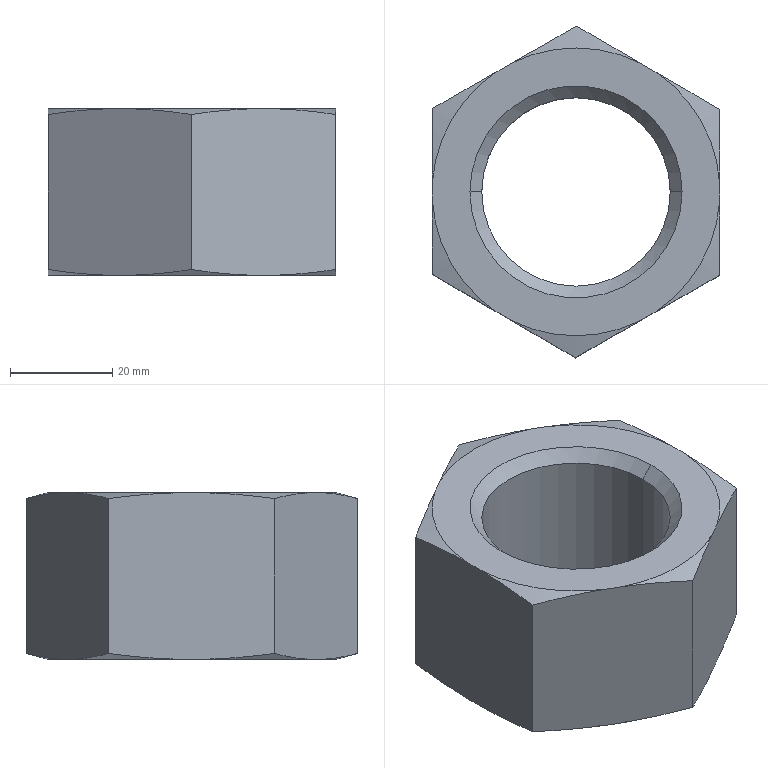Part | SolidWorks | features Cut 2, Chamfer 1, Extrusion 1 | 1 solid | 26 faces | box 56.219 x 64.769 x 32.544 mm | volume 53250 mm3 | cone 16 | plane 8 | cylinder 2 | commonest cylinder face diameters 36.8 x2
STEP:
#1=CARTESIAN_POINT('',(-18.4,0.,30.237));
#2=VERTEX_POINT('',#1);
#3=CARTESIAN_POINT('',(18.4,0.,30.237));
#4=VERTEX_POINT('',#3);
#5=CARTESIAN_POINT('',(0.,0.,30.237));
#6=DIRECTION('',(0.,0.,1.));
#7=DIRECTION('',(-1.,0.,0.));
#8=AXIS2_PLACEMENT_3D('',#5,#6,#7);
#9=CIRCLE('',#8,18.4);
#10=EDGE_CURVE('',#2,#4,#9,.T.);
#11=ORIENTED_EDGE('',*,*,#10,.F.);
#12=CARTESIAN_POINT('',(-20.707,0.,32.544));
#13=VERTEX_POINT('',#12);
#14=CARTESIAN_POINT('',(-18.4,0.,30.237));
#15=DIRECTION('',(-0.7071,0.,0.7071));
#16=VECTOR('',#15,1000.);
#17=LINE('',#14,#16);
#18=EDGE_CURVE('',#2,#13,#17,.T.);
#19=ORIENTED_EDGE('',*,*,#18,.T.);
#20=CARTESIAN_POINT('',(20.707,0.,32.544));
#21=VERTEX_POINT('',#20);
#22=CARTESIAN_POINT('',(0.,0.,32.544));
#23=DIRECTION('',(0.,0.,-1.));
#24=DIRECTION('',(-1.,0.,0.));
#25=AXIS2_PLACEMENT_3D('',#22,#23,#24);
#26=CIRCLE('',#25,20.707);
#27=EDGE_CURVE('',#21,#13,#26,.T.);
#28=ORIENTED_EDGE('',*,*,#27,.F.);
#29=CARTESIAN_POINT('',(18.4,0.,30.237));
#30=DIRECTION('',(0.7071,0.,0.7071));
#31=VECTOR('',#30,1000.);
#32=LINE('',#29,#31);
#33=EDGE_CURVE('',#4,#21,#32,.T.);
#34=ORIENTED_EDGE('',*,*,#33,.F.);
#35=EDGE_LOOP('',(#11,#19,#28,#34));
#36=FACE_OUTER_BOUND('',#35,.T.);
#37=CARTESIAN_POINT('',(0.,0.,30.237));
#38=DIRECTION('',(0.,0.,1.));
#39=DIRECTION('',(1.,0.,0.));
#40=AXIS2_PLACEMENT_3D('',#37,#38,#39);
#41=CONICAL_SURFACE('',#40,18.4,0.7854);
#42=ADVANCED_FACE('',(#36),#41,.F.);
#43=CARTESIAN_POINT('',(18.4,0.,2.307));
#44=VERTEX_POINT('',#43);
#45=CARTESIAN_POINT('',(-18.4,0.,2.307));
#46=VERTEX_POINT('',#45);
#47=CARTESIAN_POINT('',(0.,0.,2.307));
#48=DIRECTION('',(0.,0.,-1.));
#49=DIRECTION('',(-1.,0.,0.));
#50=AXIS2_PLACEMENT_3D('',#47,#48,#49);
#51=CIRCLE('',#50,18.4);
#52=EDGE_CURVE('',#44,#46,#51,.T.);
#53=ORIENTED_EDGE('',*,*,#52,.F.);
#54=CARTESIAN_POINT('',(20.707,0.,0.));
#55=VERTEX_POINT('',#54);
#56=CARTESIAN_POINT('',(20.707,0.,0.));
#57=DIRECTION('',(0.7071,0.,-0.7071));
#58=VECTOR('',#57,1000.);
#59=LINE('',#56,#58);
#60=EDGE_CURVE('',#44,#55,#59,.T.);
#61=ORIENTED_EDGE('',*,*,#60,.T.);
#62=CARTESIAN_POINT('',(-20.707,0.,0.));
#63=VERTEX_POINT('',#62);
#64=CARTESIAN_POINT('',(0.,0.,0.));
#65=DIRECTION('',(0.,0.,1.));
#66=DIRECTION('',(-1.,0.,0.));
#67=AXIS2_PLACEMENT_3D('',#64,#65,#66);
#68=CIRCLE('',#67,20.707);
#69=EDGE_CURVE('',#63,#55,#68,.T.);
#70=ORIENTED_EDGE('',*,*,#69,.F.);
#71=CARTESIAN_POINT('',(-20.707,0.,0.));
#72=DIRECTION('',(-0.7071,0.,-0.7071));
#73=VECTOR('',#72,1000.);
#74=LINE('',#71,#73);
#75=EDGE_CURVE('',#46,#63,#74,.T.);
#76=ORIENTED_EDGE('',*,*,#75,.F.);
#77=EDGE_LOOP('',(#53,#61,#70,#76));
#78=FACE_OUTER_BOUND('',#77,.T.);
#79=CARTESIAN_POINT('',(0.,0.,0.));
#80=DIRECTION('',(0.,0.,-1.));
#81=DIRECTION('',(-1.,0.,0.));
#82=AXIS2_PLACEMENT_3D('',#79,#80,#81);
#83=CONICAL_SURFACE('',#82,20.707,0.7854);
#84=ADVANCED_FACE('',(#78),#83,.F.);
#85=ORIENTED_EDGE('',*,*,#10,.T.);
#86=CARTESIAN_POINT('',(18.4,0.,32.544));
#87=DIRECTION('',(0.,0.,-1.));
#88=VECTOR('',#87,1000.);
#89=LINE('',#86,#88);
#90=EDGE_CURVE('',#4,#44,#89,.T.);
#91=ORIENTED_EDGE('',*,*,#90,.T.);
#92=ORIENTED_EDGE('',*,*,#52,.T.);
#93=CARTESIAN_POINT('',(-18.4,0.,32.544));
#94=DIRECTION('',(0.,0.,-1.));
#95=VECTOR('',#94,1000.);
#96=LINE('',#93,#95);
#97=EDGE_CURVE('',#2,#46,#96,.T.);
#98=ORIENTED_EDGE('',*,*,#97,.F.);
#99=EDGE_LOOP('',(#85,#91,#92,#98));
#100=FACE_OUTER_BOUND('',#99,.T.);
#101=CARTESIAN_POINT('',(0.,0.,32.544));
#102=DIRECTION('',(0.,0.,-1.));
#103=DIRECTION('',(-1.,0.,0.));
#104=AXIS2_PLACEMENT_3D('',#101,#102,#103);
#105=CYLINDRICAL_SURFACE('',#104,18.4);
#106=ADVANCED_FACE('',(#100),#105,.F.);
#107=CARTESIAN_POINT('',(28.11,16.082,31.396));
#108=VERTEX_POINT('',#107);
#109=CARTESIAN_POINT('',(15.62,23.359,32.544));
#110=VERTEX_POINT('',#109);
#111=CARTESIAN_POINT('',(28.11,16.082,31.396));
#112=CARTESIAN_POINT('',(26.042,17.287,31.716));
#113=CARTESIAN_POINT('',(23.968,18.495,31.984));
#114=CARTESIAN_POINT('',(19.806,20.92,32.378));
#115=CARTESIAN_POINT('',(17.718,22.137,32.504));
#116=CARTESIAN_POINT('',(15.62,23.359,32.544));
#117=B_SPLINE_CURVE_WITH_KNOTS('',3,(#111,#112,#113,#114,#115,#116),.UNSPECIFIED.,.F.,.F.,(4,2,4),(0.03192,0.03916,0.04641),.UNSPECIFIED.);
#118=EDGE_CURVE('',#108,#110,#117,.T.);
#119=ORIENTED_EDGE('',*,*,#118,.F.);
#120=CARTESIAN_POINT('',(28.11,16.082,1.148));
#121=VERTEX_POINT('',#120);
#122=CARTESIAN_POINT('',(28.11,16.082,32.544));
#123=DIRECTION('',(0.,0.,-1.));
#124=VECTOR('',#123,1000.);
#125=LINE('',#122,#124);
#126=EDGE_CURVE('',#108,#121,#125,.T.);
#127=ORIENTED_EDGE('',*,*,#126,.T.);
#128=CARTESIAN_POINT('',(15.62,23.359,0.));
#129=VERTEX_POINT('',#128);
#130=CARTESIAN_POINT('',(15.62,23.359,0.));
#131=CARTESIAN_POINT('',(16.657,22.754,0.0199));
#132=CARTESIAN_POINT('',(17.697,22.148,0.06046));
#133=CARTESIAN_POINT('',(19.781,20.934,0.1815));
#134=CARTESIAN_POINT('',(20.826,20.325,0.2621));
#135=CARTESIAN_POINT('',(23.961,18.499,0.5582));
#136=CARTESIAN_POINT('',(26.039,17.288,0.8271));
#137=CARTESIAN_POINT('',(28.11,16.082,1.148));
#138=B_SPLINE_CURVE_WITH_KNOTS('',3,(#130,#131,#132,#133,#134,#135,#136,#137),.UNSPECIFIED.,.F.,.F.,(4,2,2,4),(0.04982,0.05339,0.05695,0.06409),.UNSPECIFIED.);
#139=EDGE_CURVE('',#129,#121,#138,.T.);
#140=ORIENTED_EDGE('',*,*,#139,.F.);
#141=CARTESIAN_POINT('',(12.617,25.108,0.));
#142=VERTEX_POINT('',#141);
#143=CARTESIAN_POINT('',(28.11,16.082,0.));
#144=DIRECTION('',(-0.8641,0.5034,0.));
#145=VECTOR('',#144,1000.);
#146=LINE('',#143,#145);
#147=EDGE_CURVE('',#129,#142,#146,.T.);
#148=ORIENTED_EDGE('',*,*,#147,.T.);
#149=CARTESIAN_POINT('',(0.1274,32.385,1.148));
#150=VERTEX_POINT('',#149);
#151=CARTESIAN_POINT('',(0.1274,32.385,1.148));
#152=CARTESIAN_POINT('',(2.195,31.18,0.8275));
#153=CARTESIAN_POINT('',(4.269,29.972,0.5593));
#154=CARTESIAN_POINT('',(8.431,27.547,0.1653));
#155=CARTESIAN_POINT('',(10.519,26.33,0.04022));
#156=CARTESIAN_POINT('',(12.617,25.108,0.));
#157=B_SPLINE_CURVE_WITH_KNOTS('',3,(#151,#152,#153,#154,#155,#156),.UNSPECIFIED.,.F.,.F.,(4,2,4),(0.03188,0.03913,0.04637),.UNSPECIFIED.);
#158=EDGE_CURVE('',#150,#142,#157,.T.);
#159=ORIENTED_EDGE('',*,*,#158,.F.);
#160=CARTESIAN_POINT('',(0.1274,32.385,31.396));
#161=VERTEX_POINT('',#160);
#162=CARTESIAN_POINT('',(0.1274,32.385,32.544));
#163=DIRECTION('',(0.,0.,-1.));
#164=VECTOR('',#163,1000.);
#165=LINE('',#162,#164);
#166=EDGE_CURVE('',#161,#150,#165,.T.);
#167=ORIENTED_EDGE('',*,*,#166,.F.);
#168=CARTESIAN_POINT('',(12.617,25.108,32.544));
#169=VERTEX_POINT('',#168);
#170=CARTESIAN_POINT('',(12.617,25.108,32.544));
#171=CARTESIAN_POINT('',(11.58,25.713,32.524));
#172=CARTESIAN_POINT('',(10.54,26.318,32.483));
#173=CARTESIAN_POINT('',(8.456,27.532,32.362));
#174=CARTESIAN_POINT('',(7.411,28.141,32.282));
#175=CARTESIAN_POINT('',(4.277,29.967,31.986));
#176=CARTESIAN_POINT('',(2.198,31.178,31.717));
#177=CARTESIAN_POINT('',(0.1274,32.385,31.396));
#178=B_SPLINE_CURVE_WITH_KNOTS('',3,(#170,#171,#172,#173,#174,#175,#176,#177),.UNSPECIFIED.,.F.,.F.,(4,2,2,4),(0.04985,0.05342,0.05699,0.06413),.UNSPECIFIED.);
#179=EDGE_CURVE('',#169,#161,#178,.T.);
#180=ORIENTED_EDGE('',*,*,#179,.F.);
#181=CARTESIAN_POINT('',(28.11,16.082,32.544));
#182=DIRECTION('',(-0.8641,0.5034,0.));
#183=VECTOR('',#182,1000.);
#184=LINE('',#181,#183);
#185=EDGE_CURVE('',#110,#169,#184,.T.);
#186=ORIENTED_EDGE('',*,*,#185,.F.);
#187=EDGE_LOOP('',(#119,#127,#140,#148,#159,#167,#180,#186));
#188=FACE_OUTER_BOUND('',#187,.T.);
#189=CARTESIAN_POINT('',(28.11,16.082,32.544));
#190=DIRECTION('',(-0.5034,-0.8641,0.));
#191=DIRECTION('',(0.8641,-0.5034,0.));
#192=AXIS2_PLACEMENT_3D('',#189,#190,#191);
#193=PLANE('',#192);
#194=ADVANCED_FACE('',(#188),#193,.F.);
#195=CARTESIAN_POINT('',(-12.419,25.207,32.544));
#196=VERTEX_POINT('',#195);
#197=CARTESIAN_POINT('',(0.1274,32.385,31.396));
#198=CARTESIAN_POINT('',(-1.95,31.196,31.716));
#199=CARTESIAN_POINT('',(-4.033,30.005,31.984));
#200=CARTESIAN_POINT('',(-8.214,27.613,32.378));
#201=CARTESIAN_POINT('',(-10.312,26.412,32.504));
#202=CARTESIAN_POINT('',(-12.419,25.207,32.544));
#203=B_SPLINE_CURVE_WITH_KNOTS('',3,(#197,#198,#199,#200,#201,#202),.UNSPECIFIED.,.F.,.F.,(4,2,4),(0.03177,0.03902,0.04626),.UNSPECIFIED.);
#204=EDGE_CURVE('',#161,#196,#203,.T.);
#205=ORIENTED_EDGE('',*,*,#204,.F.);
#206=ORIENTED_EDGE('',*,*,#166,.T.);
#207=CARTESIAN_POINT('',(-12.419,25.207,0.));
#208=VERTEX_POINT('',#207);
#209=CARTESIAN_POINT('',(-12.419,25.207,0.));
#210=CARTESIAN_POINT('',(-11.377,25.803,0.0199));
#211=CARTESIAN_POINT('',(-10.333,26.4,0.06046));
#212=CARTESIAN_POINT('',(-8.239,27.598,0.1815));
#213=CARTESIAN_POINT('',(-7.189,28.199,0.262));
#214=CARTESIAN_POINT('',(-4.041,30.,0.5582));
#215=CARTESIAN_POINT('',(-1.953,31.195,0.8271));
#216=CARTESIAN_POINT('',(0.1274,32.385,1.148));
#217=B_SPLINE_CURVE_WITH_KNOTS('',3,(#209,#210,#211,#212,#213,#214,#215,#216),.UNSPECIFIED.,.F.,.F.,(4,2,2,4),(0.04967,0.05324,0.05681,0.06395),.UNSPECIFIED.);
#218=EDGE_CURVE('',#208,#150,#217,.T.);
#219=ORIENTED_EDGE('',*,*,#218,.F.);
#220=CARTESIAN_POINT('',(-15.436,23.481,0.));
#221=VERTEX_POINT('',#220);
#222=CARTESIAN_POINT('',(0.1274,32.385,0.));
#223=DIRECTION('',(-0.868,-0.4966,0.));
#224=VECTOR('',#223,1000.);
#225=LINE('',#222,#224);
#226=EDGE_CURVE('',#208,#221,#225,.T.);
#227=ORIENTED_EDGE('',*,*,#226,.T.);
#228=CARTESIAN_POINT('',(-27.982,16.303,1.148));
#229=VERTEX_POINT('',#228);
#230=CARTESIAN_POINT('',(-27.982,16.303,1.148));
#231=CARTESIAN_POINT('',(-25.905,17.491,0.8275));
#232=CARTESIAN_POINT('',(-23.822,18.683,0.5593));
#233=CARTESIAN_POINT('',(-19.641,21.075,0.1653));
#234=CARTESIAN_POINT('',(-17.543,22.275,0.04022));
#235=CARTESIAN_POINT('',(-15.436,23.481,0.));
#236=B_SPLINE_CURVE_WITH_KNOTS('',3,(#230,#231,#232,#233,#234,#235),.UNSPECIFIED.,.F.,.F.,(4,2,4),(0.03174,0.03898,0.04622),.UNSPECIFIED.);
#237=EDGE_CURVE('',#229,#221,#236,.T.);
#238=ORIENTED_EDGE('',*,*,#237,.F.);
#239=CARTESIAN_POINT('',(-27.982,16.303,31.396));
#240=VERTEX_POINT('',#239);
#241=CARTESIAN_POINT('',(-27.982,16.303,32.544));
#242=DIRECTION('',(0.,0.,-1.));
#243=VECTOR('',#242,1000.);
#244=LINE('',#241,#243);
#245=EDGE_CURVE('',#240,#229,#244,.T.);
#246=ORIENTED_EDGE('',*,*,#245,.F.);
#247=CARTESIAN_POINT('',(-15.436,23.481,32.544));
#248=VERTEX_POINT('',#247);
#249=CARTESIAN_POINT('',(-15.436,23.481,32.544));
#250=CARTESIAN_POINT('',(-16.478,22.885,32.524));
#251=CARTESIAN_POINT('',(-17.522,22.287,32.483));
#252=CARTESIAN_POINT('',(-19.616,21.089,32.362));
#253=CARTESIAN_POINT('',(-20.666,20.489,32.282));
#254=CARTESIAN_POINT('',(-23.814,18.687,31.986));
#255=CARTESIAN_POINT('',(-25.902,17.493,31.717));
#256=CARTESIAN_POINT('',(-27.982,16.303,31.396));
#257=B_SPLINE_CURVE_WITH_KNOTS('',3,(#249,#250,#251,#252,#253,#254,#255,#256),.UNSPECIFIED.,.F.,.F.,(4,2,2,4),(0.04971,0.05328,0.05684,0.06398),.UNSPECIFIED.);
#258=EDGE_CURVE('',#248,#240,#257,.T.);
#259=ORIENTED_EDGE('',*,*,#258,.F.);
#260=CARTESIAN_POINT('',(0.1274,32.385,32.544));
#261=DIRECTION('',(-0.868,-0.4966,0.));
#262=VECTOR('',#261,1000.);
#263=LINE('',#260,#262);
#264=EDGE_CURVE('',#196,#248,#263,.T.);
#265=ORIENTED_EDGE('',*,*,#264,.F.);
#266=EDGE_LOOP('',(#205,#206,#219,#227,#238,#246,#259,#265));
#267=FACE_OUTER_BOUND('',#266,.T.);
#268=CARTESIAN_POINT('',(0.1274,32.385,32.544));
#269=DIRECTION('',(0.4966,-0.868,0.));
#270=DIRECTION('',(0.868,0.4966,0.));
#271=AXIS2_PLACEMENT_3D('',#268,#269,#270);
#272=PLANE('',#271);
#273=ADVANCED_FACE('',(#267),#272,.F.);
#274=CARTESIAN_POINT('',(-28.039,1.848,32.544));
#275=VERTEX_POINT('',#274);
#276=CARTESIAN_POINT('',(-27.982,16.303,31.396));
#277=CARTESIAN_POINT('',(-27.992,13.908,31.716));
#278=CARTESIAN_POINT('',(-28.001,11.508,31.985));
#279=CARTESIAN_POINT('',(-28.02,6.691,32.379));
#280=CARTESIAN_POINT('',(-28.03,4.274,32.504));
#281=CARTESIAN_POINT('',(-28.039,1.848,32.544));
#282=B_SPLINE_CURVE_WITH_KNOTS('',3,(#276,#277,#278,#279,#280,#281),.UNSPECIFIED.,.F.,.F.,(4,2,4),(0.02754,0.03479,0.04203),.UNSPECIFIED.);
#283=EDGE_CURVE('',#240,#275,#282,.T.);
#284=ORIENTED_EDGE('',*,*,#283,.F.);
#285=ORIENTED_EDGE('',*,*,#245,.T.);
#286=CARTESIAN_POINT('',(-28.039,1.848,0.));
#287=VERTEX_POINT('',#286);
#288=CARTESIAN_POINT('',(-28.039,1.848,0.));
#289=CARTESIAN_POINT('',(-28.03,4.249,0.03978));
#290=CARTESIAN_POINT('',(-28.02,6.659,0.163));
#291=CARTESIAN_POINT('',(-28.001,11.496,0.5577));
#292=CARTESIAN_POINT('',(-27.992,13.904,0.8269));
#293=CARTESIAN_POINT('',(-27.982,16.303,1.148));
#294=B_SPLINE_CURVE_WITH_KNOTS('',3,(#288,#289,#290,#291,#292,#293),.UNSPECIFIED.,.F.,.F.,(4,2,4),(0.04546,0.0526,0.05974),.UNSPECIFIED.);
#295=EDGE_CURVE('',#287,#229,#294,.T.);
#296=ORIENTED_EDGE('',*,*,#295,.F.);
#297=CARTESIAN_POINT('',(-28.053,-1.627,0.));
#298=VERTEX_POINT('',#297);
#299=CARTESIAN_POINT('',(-27.982,16.303,0.));
#300=DIRECTION('',(-0.003934,-1.,0.));
#301=VECTOR('',#300,1000.);
#302=LINE('',#299,#301);
#303=EDGE_CURVE('',#287,#298,#302,.T.);
#304=ORIENTED_EDGE('',*,*,#303,.T.);
#305=CARTESIAN_POINT('',(-28.11,-16.082,1.148));
#306=VERTEX_POINT('',#305);
#307=CARTESIAN_POINT('',(-28.11,-16.082,1.148));
#308=CARTESIAN_POINT('',(-28.1,-13.687,0.8274));
#309=CARTESIAN_POINT('',(-28.091,-11.287,0.5591));
#310=CARTESIAN_POINT('',(-28.072,-6.47,0.1652));
#311=CARTESIAN_POINT('',(-28.062,-4.053,0.0402));
#312=CARTESIAN_POINT('',(-28.053,-1.627,0.));
#313=B_SPLINE_CURVE_WITH_KNOTS('',3,(#307,#308,#309,#310,#311,#312),.UNSPECIFIED.,.F.,.F.,(4,2,4),(0.02751,0.03476,0.042),.UNSPECIFIED.);
#314=EDGE_CURVE('',#306,#298,#313,.T.);
#315=ORIENTED_EDGE('',*,*,#314,.F.);
#316=CARTESIAN_POINT('',(-28.11,-16.082,31.396));
#317=VERTEX_POINT('',#316);
#318=CARTESIAN_POINT('',(-28.11,-16.082,32.544));
#319=DIRECTION('',(0.,0.,-1.));
#320=VECTOR('',#319,1000.);
#321=LINE('',#318,#320);
#322=EDGE_CURVE('',#317,#306,#321,.T.);
#323=ORIENTED_EDGE('',*,*,#322,.F.);
#324=CARTESIAN_POINT('',(-28.053,-1.627,32.544));
#325=VERTEX_POINT('',#324);
#326=CARTESIAN_POINT('',(-28.053,-1.627,32.544));
#327=CARTESIAN_POINT('',(-28.062,-4.028,32.504));
#328=CARTESIAN_POINT('',(-28.072,-6.438,32.381));
#329=CARTESIAN_POINT('',(-28.091,-11.275,31.986));
#330=CARTESIAN_POINT('',(-28.1,-13.684,31.717));
#331=CARTESIAN_POINT('',(-28.11,-16.082,31.396));
#332=B_SPLINE_CURVE_WITH_KNOTS('',3,(#326,#327,#328,#329,#330,#331),.UNSPECIFIED.,.F.,.F.,(4,2,4),(0.04549,0.05263,0.05977),.UNSPECIFIED.);
#333=EDGE_CURVE('',#325,#317,#332,.T.);
#334=ORIENTED_EDGE('',*,*,#333,.F.);
#335=CARTESIAN_POINT('',(-27.982,16.303,32.544));
#336=DIRECTION('',(-0.003934,-1.,0.));
#337=VECTOR('',#336,1000.);
#338=LINE('',#335,#337);
#339=EDGE_CURVE('',#275,#325,#338,.T.);
#340=ORIENTED_EDGE('',*,*,#339,.F.);
#341=EDGE_LOOP('',(#284,#285,#296,#304,#315,#323,#334,#340));
#342=FACE_OUTER_BOUND('',#341,.T.);
#343=CARTESIAN_POINT('',(-27.982,16.303,32.544));
#344=DIRECTION('',(1.,-0.003934,0.));
#345=DIRECTION('',(0.003934,1.,0.));
#346=AXIS2_PLACEMENT_3D('',#343,#344,#345);
#347=PLANE('',#346);
#348=ADVANCED_FACE('',(#342),#347,.F.);
#349=CARTESIAN_POINT('',(-15.62,-23.359,32.544));
#350=VERTEX_POINT('',#349);
#351=CARTESIAN_POINT('',(-28.11,-16.082,31.396));
#352=CARTESIAN_POINT('',(-26.042,-17.287,31.716));
#353=CARTESIAN_POINT('',(-23.968,-18.495,31.984));
#354=CARTESIAN_POINT('',(-19.806,-20.92,32.378));
#355=CARTESIAN_POINT('',(-17.718,-22.137,32.504));
#356=CARTESIAN_POINT('',(-15.62,-23.359,32.544));
#357=B_SPLINE_CURVE_WITH_KNOTS('',3,(#351,#352,#353,#354,#355,#356),.UNSPECIFIED.,.F.,.F.,(4,2,4),(0.03192,0.03916,0.04641),.UNSPECIFIED.);
#358=EDGE_CURVE('',#317,#350,#357,.T.);
#359=ORIENTED_EDGE('',*,*,#358,.F.);
#360=ORIENTED_EDGE('',*,*,#322,.T.);
#361=CARTESIAN_POINT('',(-15.62,-23.359,0.));
#362=VERTEX_POINT('',#361);
#363=CARTESIAN_POINT('',(-15.62,-23.359,0.));
#364=CARTESIAN_POINT('',(-16.657,-22.754,0.0199));
#365=CARTESIAN_POINT('',(-17.697,-22.148,0.06046));
#366=CARTESIAN_POINT('',(-19.781,-20.934,0.1815));
#367=CARTESIAN_POINT('',(-20.826,-20.325,0.2621));
#368=CARTESIAN_POINT('',(-23.961,-18.499,0.5582));
#369=CARTESIAN_POINT('',(-26.039,-17.288,0.8271));
#370=CARTESIAN_POINT('',(-28.11,-16.082,1.148));
#371=B_SPLINE_CURVE_WITH_KNOTS('',3,(#363,#364,#365,#366,#367,#368,#369,#370),.UNSPECIFIED.,.F.,.F.,(4,2,2,4),(0.04982,0.05339,0.05695,0.06409),.UNSPECIFIED.);
#372=EDGE_CURVE('',#362,#306,#371,.T.);
#373=ORIENTED_EDGE('',*,*,#372,.F.);
#374=CARTESIAN_POINT('',(-12.617,-25.108,0.));
#375=VERTEX_POINT('',#374);
#376=CARTESIAN_POINT('',(-28.11,-16.082,0.));
#377=DIRECTION('',(0.8641,-0.5034,0.));
#378=VECTOR('',#377,1000.);
#379=LINE('',#376,#378);
#380=EDGE_CURVE('',#362,#375,#379,.T.);
#381=ORIENTED_EDGE('',*,*,#380,.T.);
#382=CARTESIAN_POINT('',(-0.1274,-32.385,1.148));
#383=VERTEX_POINT('',#382);
#384=CARTESIAN_POINT('',(-0.1274,-32.385,1.148));
#385=CARTESIAN_POINT('',(-2.195,-31.18,0.8275));
#386=CARTESIAN_POINT('',(-4.269,-29.972,0.5593));
#387=CARTESIAN_POINT('',(-8.431,-27.547,0.1653));
#388=CARTESIAN_POINT('',(-10.519,-26.33,0.04022));
#389=CARTESIAN_POINT('',(-12.617,-25.108,0.));
#390=B_SPLINE_CURVE_WITH_KNOTS('',3,(#384,#385,#386,#387,#388,#389),.UNSPECIFIED.,.F.,.F.,(4,2,4),(0.03188,0.03913,0.04637),.UNSPECIFIED.);
#391=EDGE_CURVE('',#383,#375,#390,.T.);
#392=ORIENTED_EDGE('',*,*,#391,.F.);
#393=CARTESIAN_POINT('',(-0.1274,-32.385,31.396));
#394=VERTEX_POINT('',#393);
#395=CARTESIAN_POINT('',(-0.1274,-32.385,32.544));
#396=DIRECTION('',(0.,0.,-1.));
#397=VECTOR('',#396,1000.);
#398=LINE('',#395,#397);
#399=EDGE_CURVE('',#394,#383,#398,.T.);
#400=ORIENTED_EDGE('',*,*,#399,.F.);
#401=CARTESIAN_POINT('',(-12.617,-25.108,32.544));
#402=VERTEX_POINT('',#401);
#403=CARTESIAN_POINT('',(-12.617,-25.108,32.544));
#404=CARTESIAN_POINT('',(-11.58,-25.713,32.524));
#405=CARTESIAN_POINT('',(-10.54,-26.318,32.483));
#406=CARTESIAN_POINT('',(-8.456,-27.532,32.362));
#407=CARTESIAN_POINT('',(-7.411,-28.141,32.282));
#408=CARTESIAN_POINT('',(-4.277,-29.967,31.986));
#409=CARTESIAN_POINT('',(-2.198,-31.178,31.717));
#410=CARTESIAN_POINT('',(-0.1274,-32.385,31.396));
#411=B_SPLINE_CURVE_WITH_KNOTS('',3,(#403,#404,#405,#406,#407,#408,#409,#410),.UNSPECIFIED.,.F.,.F.,(4,2,2,4),(0.04985,0.05342,0.05699,0.06413),.UNSPECIFIED.);
#412=EDGE_CURVE('',#402,#394,#411,.T.);
#413=ORIENTED_EDGE('',*,*,#412,.F.);
#414=CARTESIAN_POINT('',(-28.11,-16.082,32.544));
#415=DIRECTION('',(0.8641,-0.5034,0.));
#416=VECTOR('',#415,1000.);
#417=LINE('',#414,#416);
#418=EDGE_CURVE('',#350,#402,#417,.T.);
#419=ORIENTED_EDGE('',*,*,#418,.F.);
#420=EDGE_LOOP('',(#359,#360,#373,#381,#392,#400,#413,#419));
#421=FACE_OUTER_BOUND('',#420,.T.);
#422=CARTESIAN_POINT('',(-28.11,-16.082,32.544));
#423=DIRECTION('',(0.5034,0.8641,0.));
#424=DIRECTION('',(-0.8641,0.5034,0.));
#425=AXIS2_PLACEMENT_3D('',#422,#423,#424);
#426=PLANE('',#425);
#427=ADVANCED_FACE('',(#421),#426,.F.);
#428=CARTESIAN_POINT('',(12.419,-25.207,32.544));
#429=VERTEX_POINT('',#428);
#430=CARTESIAN_POINT('',(-0.1274,-32.385,31.396));
#431=CARTESIAN_POINT('',(1.95,-31.196,31.716));
#432=CARTESIAN_POINT('',(4.033,-30.005,31.984));
#433=CARTESIAN_POINT('',(8.214,-27.613,32.378));
#434=CARTESIAN_POINT('',(10.312,-26.412,32.504));
#435=CARTESIAN_POINT('',(12.419,-25.207,32.544));
#436=B_SPLINE_CURVE_WITH_KNOTS('',3,(#430,#431,#432,#433,#434,#435),.UNSPECIFIED.,.F.,.F.,(4,2,4),(0.03177,0.03902,0.04626),.UNSPECIFIED.);
#437=EDGE_CURVE('',#394,#429,#436,.T.);
#438=ORIENTED_EDGE('',*,*,#437,.F.);
#439=ORIENTED_EDGE('',*,*,#399,.T.);
#440=CARTESIAN_POINT('',(12.419,-25.207,0.));
#441=VERTEX_POINT('',#440);
#442=CARTESIAN_POINT('',(12.419,-25.207,0.));
#443=CARTESIAN_POINT('',(11.377,-25.803,0.0199));
#444=CARTESIAN_POINT('',(10.333,-26.4,0.06046));
#445=CARTESIAN_POINT('',(8.239,-27.598,0.1815));
#446=CARTESIAN_POINT('',(7.189,-28.199,0.262));
#447=CARTESIAN_POINT('',(4.041,-30.,0.5582));
#448=CARTESIAN_POINT('',(1.953,-31.195,0.8271));
#449=CARTESIAN_POINT('',(-0.1274,-32.385,1.148));
#450=B_SPLINE_CURVE_WITH_KNOTS('',3,(#442,#443,#444,#445,#446,#447,#448,#449),.UNSPECIFIED.,.F.,.F.,(4,2,2,4),(0.04967,0.05324,0.05681,0.06395),.UNSPECIFIED.);
#451=EDGE_CURVE('',#441,#383,#450,.T.);
#452=ORIENTED_EDGE('',*,*,#451,.F.);
#453=CARTESIAN_POINT('',(15.436,-23.481,0.));
#454=VERTEX_POINT('',#453);
#455=CARTESIAN_POINT('',(-0.1274,-32.385,0.));
#456=DIRECTION('',(0.868,0.4966,0.));
#457=VECTOR('',#456,1000.);
#458=LINE('',#455,#457);
#459=EDGE_CURVE('',#441,#454,#458,.T.);
#460=ORIENTED_EDGE('',*,*,#459,.T.);
#461=CARTESIAN_POINT('',(27.982,-16.303,1.148));
#462=VERTEX_POINT('',#461);
#463=CARTESIAN_POINT('',(27.982,-16.303,1.148));
#464=CARTESIAN_POINT('',(25.905,-17.491,0.8275));
#465=CARTESIAN_POINT('',(23.822,-18.683,0.5593));
#466=CARTESIAN_POINT('',(19.641,-21.075,0.1653));
#467=CARTESIAN_POINT('',(17.543,-22.275,0.04022));
#468=CARTESIAN_POINT('',(15.436,-23.481,0.));
#469=B_SPLINE_CURVE_WITH_KNOTS('',3,(#463,#464,#465,#466,#467,#468),.UNSPECIFIED.,.F.,.F.,(4,2,4),(0.03174,0.03898,0.04622),.UNSPECIFIED.);
#470=EDGE_CURVE('',#462,#454,#469,.T.);
#471=ORIENTED_EDGE('',*,*,#470,.F.);
#472=CARTESIAN_POINT('',(27.982,-16.303,31.396));
#473=VERTEX_POINT('',#472);
#474=CARTESIAN_POINT('',(27.982,-16.303,32.544));
#475=DIRECTION('',(0.,0.,-1.));
#476=VECTOR('',#475,1000.);
#477=LINE('',#474,#476);
#478=EDGE_CURVE('',#473,#462,#477,.T.);
#479=ORIENTED_EDGE('',*,*,#478,.F.);
#480=CARTESIAN_POINT('',(15.436,-23.481,32.544));
#481=VERTEX_POINT('',#480);
#482=CARTESIAN_POINT('',(15.436,-23.481,32.544));
#483=CARTESIAN_POINT('',(16.478,-22.885,32.524));
#484=CARTESIAN_POINT('',(17.522,-22.287,32.483));
#485=CARTESIAN_POINT('',(19.616,-21.089,32.362));
#486=CARTESIAN_POINT('',(20.666,-20.489,32.282));
#487=CARTESIAN_POINT('',(23.814,-18.687,31.986));
#488=CARTESIAN_POINT('',(25.902,-17.493,31.717));
#489=CARTESIAN_POINT('',(27.982,-16.303,31.396));
#490=B_SPLINE_CURVE_WITH_KNOTS('',3,(#482,#483,#484,#485,#486,#487,#488,#489),.UNSPECIFIED.,.F.,.F.,(4,2,2,4),(0.04971,0.05328,0.05684,0.06398),.UNSPECIFIED.);
#491=EDGE_CURVE('',#481,#473,#490,.T.);
#492=ORIENTED_EDGE('',*,*,#491,.F.);
#493=CARTESIAN_POINT('',(-0.1274,-32.385,32.544));
#494=DIRECTION('',(0.868,0.4966,0.));
#495=VECTOR('',#494,1000.);
#496=LINE('',#493,#495);
#497=EDGE_CURVE('',#429,#481,#496,.T.);
#498=ORIENTED_EDGE('',*,*,#497,.F.);
#499=EDGE_LOOP('',(#438,#439,#452,#460,#471,#479,#492,#498));
#500=FACE_OUTER_BOUND('',#499,.T.);
#501=CARTESIAN_POINT('',(-0.1274,-32.385,32.544));
#502=DIRECTION('',(-0.4966,0.868,0.));
#503=DIRECTION('',(-0.868,-0.4966,0.));
#504=AXIS2_PLACEMENT_3D('',#501,#502,#503);
#505=PLANE('',#504);
#506=ADVANCED_FACE('',(#500),#505,.F.);
#507=CARTESIAN_POINT('',(28.039,-1.848,32.544));
#508=VERTEX_POINT('',#507);
#509=CARTESIAN_POINT('',(27.982,-16.303,31.396));
#510=CARTESIAN_POINT('',(27.992,-13.908,31.716));
#511=CARTESIAN_POINT('',(28.001,-11.508,31.985));
#512=CARTESIAN_POINT('',(28.02,-6.691,32.379));
#513=CARTESIAN_POINT('',(28.03,-4.274,32.504));
#514=CARTESIAN_POINT('',(28.039,-1.848,32.544));
#515=B_SPLINE_CURVE_WITH_KNOTS('',3,(#509,#510,#511,#512,#513,#514),.UNSPECIFIED.,.F.,.F.,(4,2,4),(0.02754,0.03479,0.04203),.UNSPECIFIED.);
#516=EDGE_CURVE('',#473,#508,#515,.T.);
#517=ORIENTED_EDGE('',*,*,#516,.F.);
#518=ORIENTED_EDGE('',*,*,#478,.T.);
#519=CARTESIAN_POINT('',(28.039,-1.848,0.));
#520=VERTEX_POINT('',#519);
#521=CARTESIAN_POINT('',(28.039,-1.848,0.));
#522=CARTESIAN_POINT('',(28.03,-4.249,0.03978));
#523=CARTESIAN_POINT('',(28.02,-6.659,0.163));
#524=CARTESIAN_POINT('',(28.001,-11.496,0.5577));
#525=CARTESIAN_POINT('',(27.992,-13.904,0.8269));
#526=CARTESIAN_POINT('',(27.982,-16.303,1.148));
#527=B_SPLINE_CURVE_WITH_KNOTS('',3,(#521,#522,#523,#524,#525,#526),.UNSPECIFIED.,.F.,.F.,(4,2,4),(0.04546,0.0526,0.05974),.UNSPECIFIED.);
#528=EDGE_CURVE('',#520,#462,#527,.T.);
#529=ORIENTED_EDGE('',*,*,#528,.F.);
#530=CARTESIAN_POINT('',(28.053,1.627,0.));
#531=VERTEX_POINT('',#530);
#532=CARTESIAN_POINT('',(27.982,-16.303,0.));
#533=DIRECTION('',(0.003934,1.,0.));
#534=VECTOR('',#533,1000.);
#535=LINE('',#532,#534);
#536=EDGE_CURVE('',#520,#531,#535,.T.);
#537=ORIENTED_EDGE('',*,*,#536,.T.);
#538=CARTESIAN_POINT('',(28.11,16.082,1.148));
#539=CARTESIAN_POINT('',(28.1,13.687,0.8274));
#540=CARTESIAN_POINT('',(28.091,11.287,0.5591));
#541=CARTESIAN_POINT('',(28.072,6.47,0.1652));
#542=CARTESIAN_POINT('',(28.062,4.053,0.0402));
#543=CARTESIAN_POINT('',(28.053,1.627,0.));
#544=B_SPLINE_CURVE_WITH_KNOTS('',3,(#538,#539,#540,#541,#542,#543),.UNSPECIFIED.,.F.,.F.,(4,2,4),(0.02751,0.03476,0.042),.UNSPECIFIED.);
#545=EDGE_CURVE('',#121,#531,#544,.T.);
#546=ORIENTED_EDGE('',*,*,#545,.F.);
#547=ORIENTED_EDGE('',*,*,#126,.F.);
#548=CARTESIAN_POINT('',(28.053,1.627,32.544));
#549=VERTEX_POINT('',#548);
#550=CARTESIAN_POINT('',(28.053,1.627,32.544));
#551=CARTESIAN_POINT('',(28.062,4.028,32.504));
#552=CARTESIAN_POINT('',(28.072,6.438,32.381));
#553=CARTESIAN_POINT('',(28.091,11.275,31.986));
#554=CARTESIAN_POINT('',(28.1,13.684,31.717));
#555=CARTESIAN_POINT('',(28.11,16.082,31.396));
#556=B_SPLINE_CURVE_WITH_KNOTS('',3,(#550,#551,#552,#553,#554,#555),.UNSPECIFIED.,.F.,.F.,(4,2,4),(0.04549,0.05263,0.05977),.UNSPECIFIED.);
#557=EDGE_CURVE('',#549,#108,#556,.T.);
#558=ORIENTED_EDGE('',*,*,#557,.F.);
#559=CARTESIAN_POINT('',(27.982,-16.303,32.544));
#560=DIRECTION('',(0.003934,1.,0.));
#561=VECTOR('',#560,1000.);
#562=LINE('',#559,#561);
#563=EDGE_CURVE('',#508,#549,#562,.T.);
#564=ORIENTED_EDGE('',*,*,#563,.F.);
#565=EDGE_LOOP('',(#517,#518,#529,#537,#546,#547,#558,#564));
#566=FACE_OUTER_BOUND('',#565,.T.);
#567=CARTESIAN_POINT('',(27.982,-16.303,32.544));
#568=DIRECTION('',(-1.,0.003934,0.));
#569=DIRECTION('',(-0.003934,-1.,0.));
#570=AXIS2_PLACEMENT_3D('',#567,#568,#569);
#571=PLANE('',#570);
#572=ADVANCED_FACE('',(#566),#571,.F.);
#573=ORIENTED_EDGE('',*,*,#27,.T.);
#574=CARTESIAN_POINT('',(0.,0.,32.544));
#575=DIRECTION('',(0.,0.,-1.));
#576=DIRECTION('',(-1.,0.,0.));
#577=AXIS2_PLACEMENT_3D('',#574,#575,#576);
#578=CIRCLE('',#577,20.707);
#579=EDGE_CURVE('',#13,#21,#578,.T.);
#580=ORIENTED_EDGE('',*,*,#579,.T.);
#581=EDGE_LOOP('',(#573,#580));
#582=FACE_BOUND('',#581,.T.);
#583=CARTESIAN_POINT('',(0.,0.,32.544));
#584=DIRECTION('',(0.,0.,-1.));
#585=DIRECTION('',(-1.,0.,0.));
#586=AXIS2_PLACEMENT_3D('',#583,#584,#585);
#587=CIRCLE('',#586,28.1);
#588=EDGE_CURVE('',#275,#248,#587,.T.);
#589=ORIENTED_EDGE('',*,*,#588,.F.);
#590=ORIENTED_EDGE('',*,*,#339,.T.);
#591=CARTESIAN_POINT('',(0.,0.,32.544));
#592=DIRECTION('',(0.,0.,-1.));
#593=DIRECTION('',(-1.,0.,0.));
#594=AXIS2_PLACEMENT_3D('',#591,#592,#593);
#595=CIRCLE('',#594,28.1);
#596=EDGE_CURVE('',#350,#325,#595,.T.);
#597=ORIENTED_EDGE('',*,*,#596,.F.);
#598=ORIENTED_EDGE('',*,*,#418,.T.);
#599=CARTESIAN_POINT('',(0.,0.,32.544));
#600=DIRECTION('',(0.,0.,-1.));
#601=DIRECTION('',(-1.,0.,0.));
#602=AXIS2_PLACEMENT_3D('',#599,#600,#601);
#603=CIRCLE('',#602,28.1);
#604=EDGE_CURVE('',#429,#402,#603,.T.);
#605=ORIENTED_EDGE('',*,*,#604,.F.);
#606=ORIENTED_EDGE('',*,*,#497,.T.);
#607=CARTESIAN_POINT('',(0.,0.,32.544));
#608=DIRECTION('',(0.,0.,-1.));
#609=DIRECTION('',(-1.,0.,0.));
#610=AXIS2_PLACEMENT_3D('',#607,#608,#609);
#611=CIRCLE('',#610,28.1);
#612=EDGE_CURVE('',#508,#481,#611,.T.);
#613=ORIENTED_EDGE('',*,*,#612,.F.);
#614=ORIENTED_EDGE('',*,*,#563,.T.);
#615=CARTESIAN_POINT('',(0.,0.,32.544));
#616=DIRECTION('',(0.,0.,1.));
#617=DIRECTION('',(1.,0.,0.));
#618=AXIS2_PLACEMENT_3D('',#615,#616,#617);
#619=CIRCLE('',#618,28.1);
#620=EDGE_CURVE('',#549,#110,#619,.T.);
#621=ORIENTED_EDGE('',*,*,#620,.T.);
#622=ORIENTED_EDGE('',*,*,#185,.T.);
#623=CARTESIAN_POINT('',(0.,0.,32.544));
#624=DIRECTION('',(0.,0.,-1.));
#625=DIRECTION('',(-1.,0.,0.));
#626=AXIS2_PLACEMENT_3D('',#623,#624,#625);
#627=CIRCLE('',#626,28.1);
#628=EDGE_CURVE('',#196,#169,#627,.T.);
#629=ORIENTED_EDGE('',*,*,#628,.F.);
#630=ORIENTED_EDGE('',*,*,#264,.T.);
#631=EDGE_LOOP('',(#589,#590,#597,#598,#605,#606,#613,#614,#621,#622,#629,#630));
#632=FACE_OUTER_BOUND('',#631,.T.);
#633=CARTESIAN_POINT('',(56.092,-0.2206,32.544));
#634=DIRECTION('',(0.,0.,-1.));
#635=DIRECTION('',(-1.,0.,0.));
#636=AXIS2_PLACEMENT_3D('',#633,#634,#635);
#637=PLANE('',#636);
#638=ADVANCED_FACE('',(#582,#632),#637,.F.);
#639=ORIENTED_EDGE('',*,*,#69,.T.);
#640=CARTESIAN_POINT('',(0.,0.,0.));
#641=DIRECTION('',(0.,0.,1.));
#642=DIRECTION('',(-1.,0.,0.));
#643=AXIS2_PLACEMENT_3D('',#640,#641,#642);
#644=CIRCLE('',#643,20.707);
#645=EDGE_CURVE('',#55,#63,#644,.T.);
#646=ORIENTED_EDGE('',*,*,#645,.T.);
#647=EDGE_LOOP('',(#639,#646));
#648=FACE_BOUND('',#647,.T.);
#649=ORIENTED_EDGE('',*,*,#303,.F.);
#650=CARTESIAN_POINT('',(0.,0.,0.));
#651=DIRECTION('',(0.,0.,-1.));
#652=DIRECTION('',(-1.,0.,0.));
#653=AXIS2_PLACEMENT_3D('',#650,#651,#652);
#654=CIRCLE('',#653,28.1);
#655=EDGE_CURVE('',#287,#221,#654,.T.);
#656=ORIENTED_EDGE('',*,*,#655,.T.);
#657=ORIENTED_EDGE('',*,*,#226,.F.);
#658=CARTESIAN_POINT('',(0.,0.,0.));
#659=DIRECTION('',(0.,0.,-1.));
#660=DIRECTION('',(-1.,0.,0.));
#661=AXIS2_PLACEMENT_3D('',#658,#659,#660);
#662=CIRCLE('',#661,28.1);
#663=EDGE_CURVE('',#208,#142,#662,.T.);
#664=ORIENTED_EDGE('',*,*,#663,.T.);
#665=ORIENTED_EDGE('',*,*,#147,.F.);
#666=CARTESIAN_POINT('',(0.,0.,0.));
#667=DIRECTION('',(0.,0.,-1.));
#668=DIRECTION('',(-1.,0.,0.));
#669=AXIS2_PLACEMENT_3D('',#666,#667,#668);
#670=CIRCLE('',#669,28.1);
#671=EDGE_CURVE('',#129,#531,#670,.T.);
#672=ORIENTED_EDGE('',*,*,#671,.T.);
#673=ORIENTED_EDGE('',*,*,#536,.F.);
#674=CARTESIAN_POINT('',(0.,0.,0.));
#675=DIRECTION('',(0.,0.,-1.));
#676=DIRECTION('',(-1.,0.,0.));
#677=AXIS2_PLACEMENT_3D('',#674,#675,#676);
#678=CIRCLE('',#677,28.1);
#679=EDGE_CURVE('',#520,#454,#678,.T.);
#680=ORIENTED_EDGE('',*,*,#679,.T.);
#681=ORIENTED_EDGE('',*,*,#459,.F.);
#682=CARTESIAN_POINT('',(0.,0.,0.));
#683=DIRECTION('',(0.,0.,-1.));
#684=DIRECTION('',(-1.,0.,0.));
#685=AXIS2_PLACEMENT_3D('',#682,#683,#684);
#686=CIRCLE('',#685,28.1);
#687=EDGE_CURVE('',#441,#375,#686,.T.);
#688=ORIENTED_EDGE('',*,*,#687,.T.);
#689=ORIENTED_EDGE('',*,*,#380,.F.);
#690=CARTESIAN_POINT('',(0.,0.,0.));
#691=DIRECTION('',(0.,0.,-1.));
#692=DIRECTION('',(-1.,0.,0.));
#693=AXIS2_PLACEMENT_3D('',#690,#691,#692);
#694=CIRCLE('',#693,28.1);
#695=EDGE_CURVE('',#362,#298,#694,.T.);
#696=ORIENTED_EDGE('',*,*,#695,.T.);
#697=EDGE_LOOP('',(#649,#656,#657,#664,#665,#672,#673,#680,#681,#688,#689,#696));
#698=FACE_OUTER_BOUND('',#697,.T.);
#699=CARTESIAN_POINT('',(56.092,-0.2206,0.));
#700=DIRECTION('',(0.,0.,-1.));
#701=DIRECTION('',(-1.,0.,0.));
#702=AXIS2_PLACEMENT_3D('',#699,#700,#701);
#703=PLANE('',#702);
#704=ADVANCED_FACE('',(#648,#698),#703,.T.);
#705=ORIENTED_EDGE('',*,*,#90,.F.);
#706=CARTESIAN_POINT('',(0.,0.,30.237));
#707=DIRECTION('',(0.,0.,1.));
#708=DIRECTION('',(-1.,0.,0.));
#709=AXIS2_PLACEMENT_3D('',#706,#707,#708);
#710=CIRCLE('',#709,18.4);
#711=EDGE_CURVE('',#4,#2,#710,.T.);
#712=ORIENTED_EDGE('',*,*,#711,.T.);
#713=ORIENTED_EDGE('',*,*,#97,.T.);
#714=CARTESIAN_POINT('',(0.,0.,2.307));
#715=DIRECTION('',(0.,0.,-1.));
#716=DIRECTION('',(-1.,0.,0.));
#717=AXIS2_PLACEMENT_3D('',#714,#715,#716);
#718=CIRCLE('',#717,18.4);
#719=EDGE_CURVE('',#46,#44,#718,.T.);
#720=ORIENTED_EDGE('',*,*,#719,.T.);
#721=EDGE_LOOP('',(#705,#712,#713,#720));
#722=FACE_OUTER_BOUND('',#721,.T.);
#723=CARTESIAN_POINT('',(0.,0.,32.544));
#724=DIRECTION('',(0.,0.,-1.));
#725=DIRECTION('',(-1.,0.,0.));
#726=AXIS2_PLACEMENT_3D('',#723,#724,#725);
#727=CYLINDRICAL_SURFACE('',#726,18.4);
#728=ADVANCED_FACE('',(#722),#727,.F.);
#729=ORIENTED_EDGE('',*,*,#470,.T.);
#730=ORIENTED_EDGE('',*,*,#679,.F.);
#731=ORIENTED_EDGE('',*,*,#528,.T.);
#732=EDGE_LOOP('',(#729,#730,#731));
#733=FACE_OUTER_BOUND('',#732,.T.);
#734=CARTESIAN_POINT('',(0.,0.,0.));
#735=DIRECTION('',(0.,0.,1.));
#736=DIRECTION('',(-1.,0.,0.));
#737=AXIS2_PLACEMENT_3D('',#734,#735,#736);
#738=CONICAL_SURFACE('',#737,28.1,1.309);
#739=ADVANCED_FACE('',(#733),#738,.T.);
#740=ORIENTED_EDGE('',*,*,#139,.T.);
#741=ORIENTED_EDGE('',*,*,#545,.T.);
#742=ORIENTED_EDGE('',*,*,#671,.F.);
#743=EDGE_LOOP('',(#740,#741,#742));
#744=FACE_OUTER_BOUND('',#743,.T.);
#745=CARTESIAN_POINT('',(0.,0.,0.));
#746=DIRECTION('',(0.,0.,1.));
#747=DIRECTION('',(-1.,0.,0.));
#748=AXIS2_PLACEMENT_3D('',#745,#746,#747);
#749=CONICAL_SURFACE('',#748,28.1,1.309);
#750=ADVANCED_FACE('',(#744),#749,.T.);
#751=ORIENTED_EDGE('',*,*,#391,.T.);
#752=ORIENTED_EDGE('',*,*,#687,.F.);
#753=ORIENTED_EDGE('',*,*,#451,.T.);
#754=EDGE_LOOP('',(#751,#752,#753));
#755=FACE_OUTER_BOUND('',#754,.T.);
#756=CARTESIAN_POINT('',(0.,0.,0.));
#757=DIRECTION('',(0.,0.,1.));
#758=DIRECTION('',(-1.,0.,0.));
#759=AXIS2_PLACEMENT_3D('',#756,#757,#758);
#760=CONICAL_SURFACE('',#759,28.1,1.309);
#761=ADVANCED_FACE('',(#755),#760,.T.);
#762=ORIENTED_EDGE('',*,*,#314,.T.);
#763=ORIENTED_EDGE('',*,*,#695,.F.);
#764=ORIENTED_EDGE('',*,*,#372,.T.);
#765=EDGE_LOOP('',(#762,#763,#764));
#766=FACE_OUTER_BOUND('',#765,.T.);
#767=CARTESIAN_POINT('',(0.,0.,0.));
#768=DIRECTION('',(0.,0.,1.));
#769=DIRECTION('',(-1.,0.,0.));
#770=AXIS2_PLACEMENT_3D('',#767,#768,#769);
#771=CONICAL_SURFACE('',#770,28.1,1.309);
#772=ADVANCED_FACE('',(#766),#771,.T.);
#773=ORIENTED_EDGE('',*,*,#237,.T.);
#774=ORIENTED_EDGE('',*,*,#655,.F.);
#775=ORIENTED_EDGE('',*,*,#295,.T.);
#776=EDGE_LOOP('',(#773,#774,#775));
#777=FACE_OUTER_BOUND('',#776,.T.);
#778=CARTESIAN_POINT('',(0.,0.,0.));
#779=DIRECTION('',(0.,0.,1.));
#780=DIRECTION('',(-1.,0.,0.));
#781=AXIS2_PLACEMENT_3D('',#778,#779,#780);
#782=CONICAL_SURFACE('',#781,28.1,1.309);
#783=ADVANCED_FACE('',(#777),#782,.T.);
#784=ORIENTED_EDGE('',*,*,#158,.T.);
#785=ORIENTED_EDGE('',*,*,#663,.F.);
#786=ORIENTED_EDGE('',*,*,#218,.T.);
#787=EDGE_LOOP('',(#784,#785,#786));
#788=FACE_OUTER_BOUND('',#787,.T.);
#789=CARTESIAN_POINT('',(0.,0.,0.));
#790=DIRECTION('',(0.,0.,1.));
#791=DIRECTION('',(-1.,0.,0.));
#792=AXIS2_PLACEMENT_3D('',#789,#790,#791);
#793=CONICAL_SURFACE('',#792,28.1,1.309);
#794=ADVANCED_FACE('',(#788),#793,.T.);
#795=ORIENTED_EDGE('',*,*,#333,.T.);
#796=ORIENTED_EDGE('',*,*,#358,.T.);
#797=ORIENTED_EDGE('',*,*,#596,.T.);
#798=EDGE_LOOP('',(#795,#796,#797));
#799=FACE_OUTER_BOUND('',#798,.T.);
#800=CARTESIAN_POINT('',(0.,0.,32.544));
#801=DIRECTION('',(0.,0.,-1.));
#802=DIRECTION('',(1.,0.,0.));
#803=AXIS2_PLACEMENT_3D('',#800,#801,#802);
#804=CONICAL_SURFACE('',#803,28.1,1.309);
#805=ADVANCED_FACE('',(#799),#804,.T.);
#806=ORIENTED_EDGE('',*,*,#412,.T.);
#807=ORIENTED_EDGE('',*,*,#437,.T.);
#808=ORIENTED_EDGE('',*,*,#604,.T.);
#809=EDGE_LOOP('',(#806,#807,#808));
#810=FACE_OUTER_BOUND('',#809,.T.);
#811=CARTESIAN_POINT('',(0.,0.,32.544));
#812=DIRECTION('',(0.,0.,-1.));
#813=DIRECTION('',(1.,0.,0.));
#814=AXIS2_PLACEMENT_3D('',#811,#812,#813);
#815=CONICAL_SURFACE('',#814,28.1,1.309);
#816=ADVANCED_FACE('',(#810),#815,.T.);
#817=ORIENTED_EDGE('',*,*,#491,.T.);
#818=ORIENTED_EDGE('',*,*,#516,.T.);
#819=ORIENTED_EDGE('',*,*,#612,.T.);
#820=EDGE_LOOP('',(#817,#818,#819));
#821=FACE_OUTER_BOUND('',#820,.T.);
#822=CARTESIAN_POINT('',(0.,0.,32.544));
#823=DIRECTION('',(0.,0.,-1.));
#824=DIRECTION('',(1.,0.,0.));
#825=AXIS2_PLACEMENT_3D('',#822,#823,#824);
#826=CONICAL_SURFACE('',#825,28.1,1.309);
#827=ADVANCED_FACE('',(#821),#826,.T.);
#828=ORIENTED_EDGE('',*,*,#118,.T.);
#829=ORIENTED_EDGE('',*,*,#620,.F.);
#830=ORIENTED_EDGE('',*,*,#557,.T.);
#831=EDGE_LOOP('',(#828,#829,#830));
#832=FACE_OUTER_BOUND('',#831,.T.);
#833=CARTESIAN_POINT('',(0.,0.,32.544));
#834=DIRECTION('',(0.,0.,-1.));
#835=DIRECTION('',(1.,0.,0.));
#836=AXIS2_PLACEMENT_3D('',#833,#834,#835);
#837=CONICAL_SURFACE('',#836,28.1,1.309);
#838=ADVANCED_FACE('',(#832),#837,.T.);
#839=ORIENTED_EDGE('',*,*,#179,.T.);
#840=ORIENTED_EDGE('',*,*,#204,.T.);
#841=ORIENTED_EDGE('',*,*,#628,.T.);
#842=EDGE_LOOP('',(#839,#840,#841));
#843=FACE_OUTER_BOUND('',#842,.T.);
#844=CARTESIAN_POINT('',(0.,0.,32.544));
#845=DIRECTION('',(0.,0.,-1.));
#846=DIRECTION('',(1.,0.,0.));
#847=AXIS2_PLACEMENT_3D('',#844,#845,#846);
#848=CONICAL_SURFACE('',#847,28.1,1.309);
#849=ADVANCED_FACE('',(#843),#848,.T.);
#850=ORIENTED_EDGE('',*,*,#258,.T.);
#851=ORIENTED_EDGE('',*,*,#283,.T.);
#852=ORIENTED_EDGE('',*,*,#588,.T.);
#853=EDGE_LOOP('',(#850,#851,#852));
#854=FACE_OUTER_BOUND('',#853,.T.);
#855=CARTESIAN_POINT('',(0.,0.,32.544));
#856=DIRECTION('',(0.,0.,-1.));
#857=DIRECTION('',(1.,0.,0.));
#858=AXIS2_PLACEMENT_3D('',#855,#856,#857);
#859=CONICAL_SURFACE('',#858,28.1,1.309);
#860=ADVANCED_FACE('',(#854),#859,.T.);
#861=ORIENTED_EDGE('',*,*,#60,.F.);
#862=ORIENTED_EDGE('',*,*,#719,.F.);
#863=ORIENTED_EDGE('',*,*,#75,.T.);
#864=ORIENTED_EDGE('',*,*,#645,.F.);
#865=EDGE_LOOP('',(#861,#862,#863,#864));
#866=FACE_OUTER_BOUND('',#865,.T.);
#867=CARTESIAN_POINT('',(0.,0.,0.));
#868=DIRECTION('',(0.,0.,-1.));
#869=DIRECTION('',(-1.,0.,0.));
#870=AXIS2_PLACEMENT_3D('',#867,#868,#869);
#871=CONICAL_SURFACE('',#870,20.707,0.7854);
#872=ADVANCED_FACE('',(#866),#871,.F.);
#873=ORIENTED_EDGE('',*,*,#18,.F.);
#874=ORIENTED_EDGE('',*,*,#711,.F.);
#875=ORIENTED_EDGE('',*,*,#33,.T.);
#876=ORIENTED_EDGE('',*,*,#579,.F.);
#877=EDGE_LOOP('',(#873,#874,#875,#876));
#878=FACE_OUTER_BOUND('',#877,.T.);
#879=CARTESIAN_POINT('',(0.,0.,30.237));
#880=DIRECTION('',(0.,0.,1.));
#881=DIRECTION('',(1.,0.,0.));
#882=AXIS2_PLACEMENT_3D('',#879,#880,#881);
#883=CONICAL_SURFACE('',#882,18.4,0.7854);
#884=ADVANCED_FACE('',(#878),#883,.F.);
#885=CLOSED_SHELL('',(#42,#84,#106,#194,#273,#348,#427,#506,#572,#638,#704,#728,#739,#750,#761,#772,#783,#794,#805,#816,#827,#838,#849,#860,#872,#884));
#886=MANIFOLD_SOLID_BREP('',#885);
#887=CARTESIAN_POINT('',(0.,0.,0.));
#888=DIRECTION('',(0.,0.,1.));
#889=DIRECTION('',(1.,0.,0.));
#890=AXIS2_PLACEMENT_3D('',#887,#888,#889);
#891=(LENGTH_UNIT()NAMED_UNIT(*)SI_UNIT(.MILLI.,.METRE.));
#892=UNCERTAINTY_MEASURE_WITH_UNIT(LENGTH_MEASURE(0.00001),#891,'','');
#893=(NAMED_UNIT(*)PLANE_ANGLE_UNIT()SI_UNIT($,.RADIAN.));
#894=(NAMED_UNIT(*)SI_UNIT($,.STERADIAN.)SOLID_ANGLE_UNIT());
#895=(GEOMETRIC_REPRESENTATION_CONTEXT(3)GLOBAL_UNCERTAINTY_ASSIGNED_CONTEXT((#892))GLOBAL_UNIT_ASSIGNED_CONTEXT((#891,#893,#894))REPRESENTATION_CONTEXT('',''));
#896=ADVANCED_BREP_SHAPE_REPRESENTATION('',(#886,#890),#895);